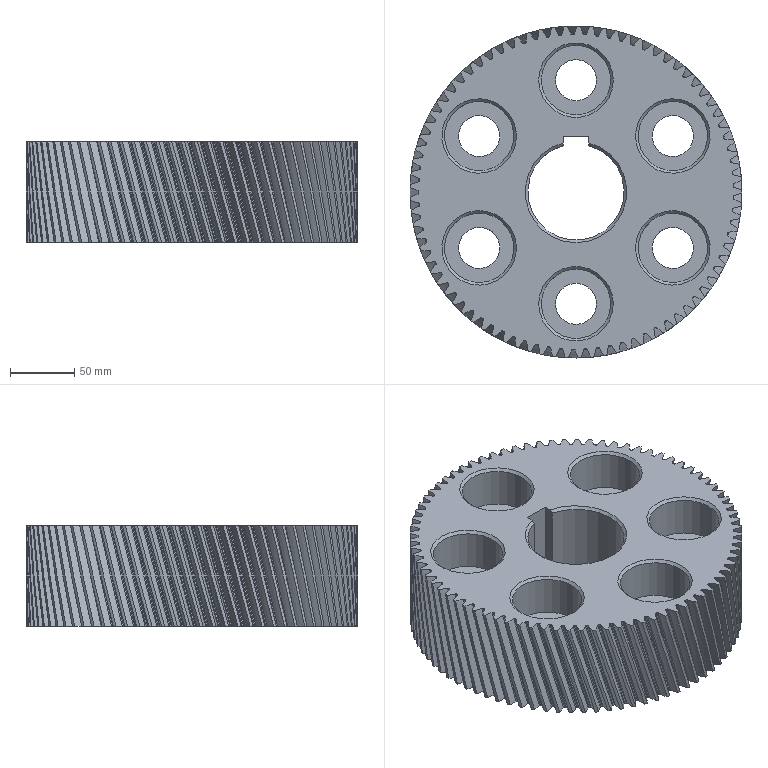Part | NX | 1 solid | 536 faces | box 258.17 x 258.17 x 78 mm | volume 2559189 mm3 | spline 405 | cylinder 100 | plane 17 | cone 14 | commonest cylinder face diameters 244.67 x81 54 x12 32 x6 75 x1